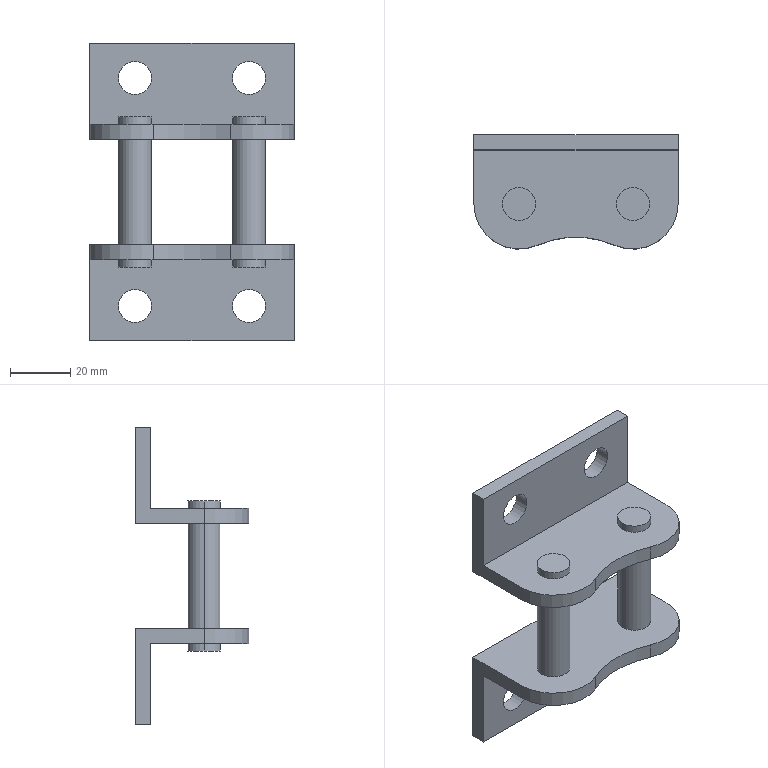Part | STEP file | 24A double-side double-hole chain 1 | 1 solid | 44 faces | box 68 x 38 x 99 mm | volume 48081 mm3 | cylinder 26 | plane 18 | commonest cylinder face diameters 11 x20 30 x4 64.25 x2